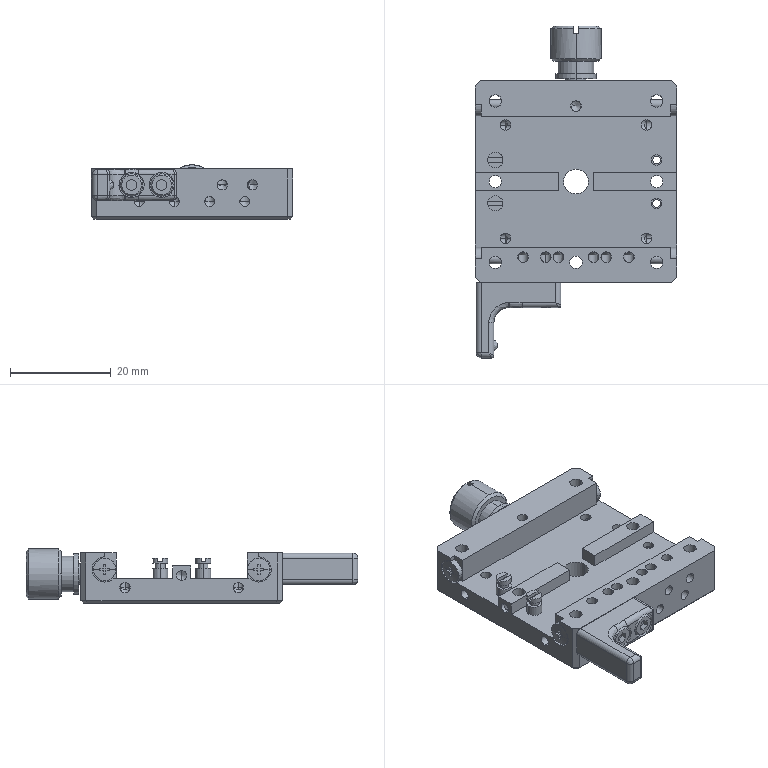Part | SolidWorks | features BaseBody 12 | 12 solids | 522 faces | box 40 x 65.9 x 10.8 mm | volume 11595 mm3 | cylinder 210 | plane 174 | cone 98 | spline 24 | torus 16 | commonest cylinder face diameters 2.1 x41 2 x39 2.013 x34 2.459 x18 3 x12 4.5 x12